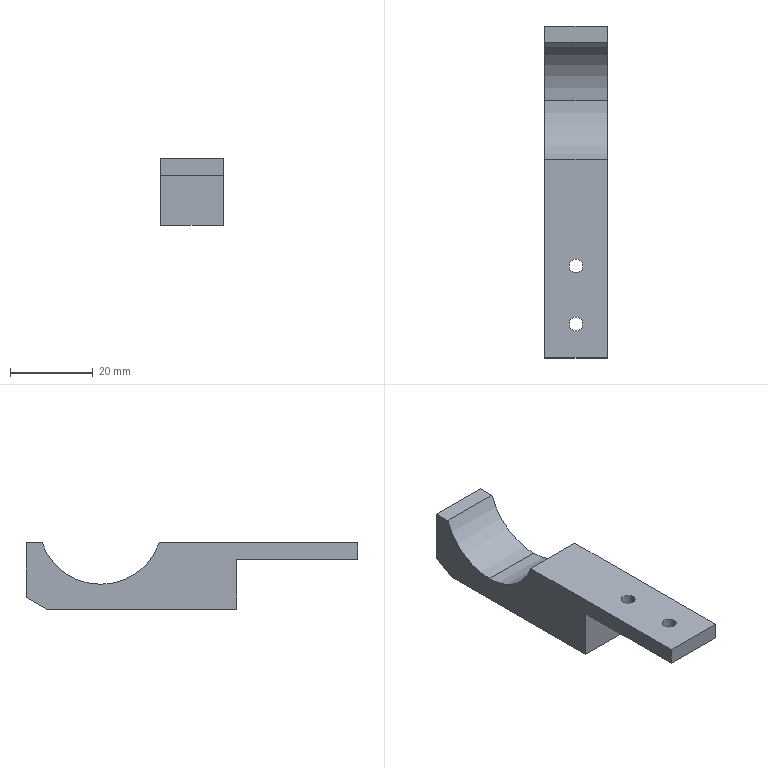Part | SolidWorks | features ICE 2, Chamfer 1, Extrusion 1, HoleWzd 1 | 1 solid | 16 faces | box 15 x 80 x 16 mm | volume 10673 mm3 | plane 10 | cylinder 6 | commonest cylinder face diameters 3.3 x4 30 x2
STEP:
#1=CARTESIAN_POINT('',(-7.5,22.,6.));
#2=VERTEX_POINT('',#1);
#3=CARTESIAN_POINT('',(-7.5,36.142,16.));
#4=VERTEX_POINT('',#3);
#5=CARTESIAN_POINT('',(-7.5,22.,21.));
#6=DIRECTION('',(1.,0.,0.));
#7=DIRECTION('',(0.,0.,-1.));
#8=AXIS2_PLACEMENT_3D('',#5,#6,#7);
#9=CIRCLE('',#8,15.);
#10=EDGE_CURVE('',#2,#4,#9,.T.);
#11=ORIENTED_EDGE('',*,*,#10,.F.);
#12=CARTESIAN_POINT('',(7.5,22.,6.));
#13=VERTEX_POINT('',#12);
#14=CARTESIAN_POINT('',(-7.5,22.,6.));
#15=DIRECTION('',(1.,0.,0.));
#16=VECTOR('',#15,1000.);
#17=LINE('',#14,#16);
#18=EDGE_CURVE('',#2,#13,#17,.T.);
#19=ORIENTED_EDGE('',*,*,#18,.T.);
#20=CARTESIAN_POINT('',(7.5,36.142,16.));
#21=VERTEX_POINT('',#20);
#22=CARTESIAN_POINT('',(7.5,22.,21.));
#23=DIRECTION('',(1.,0.,0.));
#24=DIRECTION('',(0.,0.,-1.));
#25=AXIS2_PLACEMENT_3D('',#22,#23,#24);
#26=CIRCLE('',#25,15.);
#27=EDGE_CURVE('',#13,#21,#26,.T.);
#28=ORIENTED_EDGE('',*,*,#27,.T.);
#29=CARTESIAN_POINT('',(-7.5,36.142,16.));
#30=DIRECTION('',(1.,0.,0.));
#31=VECTOR('',#30,1000.);
#32=LINE('',#29,#31);
#33=EDGE_CURVE('',#4,#21,#32,.T.);
#34=ORIENTED_EDGE('',*,*,#33,.F.);
#35=EDGE_LOOP('',(#11,#19,#28,#34));
#36=FACE_OUTER_BOUND('',#35,.T.);
#37=CARTESIAN_POINT('',(-7.5,22.,21.));
#38=DIRECTION('',(1.,0.,0.));
#39=DIRECTION('',(0.,0.,-1.));
#40=AXIS2_PLACEMENT_3D('',#37,#38,#39);
#41=CYLINDRICAL_SURFACE('',#40,15.);
#42=ADVANCED_FACE('',(#36),#41,.F.);
#43=CARTESIAN_POINT('',(1.65,-17.8,16.));
#44=VERTEX_POINT('',#43);
#45=CARTESIAN_POINT('',(-1.65,-17.8,16.));
#46=VERTEX_POINT('',#45);
#47=CARTESIAN_POINT('',(0.,-17.8,16.));
#48=DIRECTION('',(0.,0.,-1.));
#49=DIRECTION('',(-1.,0.,0.));
#50=AXIS2_PLACEMENT_3D('',#47,#48,#49);
#51=CIRCLE('',#50,1.65);
#52=EDGE_CURVE('',#44,#46,#51,.T.);
#53=ORIENTED_EDGE('',*,*,#52,.F.);
#54=CARTESIAN_POINT('',(1.65,-17.8,12.));
#55=VERTEX_POINT('',#54);
#56=CARTESIAN_POINT('',(1.65,-17.8,12.));
#57=DIRECTION('',(0.,0.,-1.));
#58=VECTOR('',#57,1000.);
#59=LINE('',#56,#58);
#60=EDGE_CURVE('',#44,#55,#59,.T.);
#61=ORIENTED_EDGE('',*,*,#60,.T.);
#62=CARTESIAN_POINT('',(-1.65,-17.8,12.));
#63=VERTEX_POINT('',#62);
#64=CARTESIAN_POINT('',(0.,-17.8,12.));
#65=DIRECTION('',(0.,0.,-1.));
#66=DIRECTION('',(-1.,0.,0.));
#67=AXIS2_PLACEMENT_3D('',#64,#65,#66);
#68=CIRCLE('',#67,1.65);
#69=EDGE_CURVE('',#55,#63,#68,.T.);
#70=ORIENTED_EDGE('',*,*,#69,.T.);
#71=CARTESIAN_POINT('',(-1.65,-17.8,12.));
#72=DIRECTION('',(0.,0.,-1.));
#73=VECTOR('',#72,1000.);
#74=LINE('',#71,#73);
#75=EDGE_CURVE('',#46,#63,#74,.T.);
#76=ORIENTED_EDGE('',*,*,#75,.F.);
#77=EDGE_LOOP('',(#53,#61,#70,#76));
#78=FACE_OUTER_BOUND('',#77,.T.);
#79=CARTESIAN_POINT('',(0.,-17.8,12.));
#80=DIRECTION('',(0.,0.,-1.));
#81=DIRECTION('',(-1.,0.,0.));
#82=AXIS2_PLACEMENT_3D('',#79,#80,#81);
#83=CYLINDRICAL_SURFACE('',#82,1.65);
#84=ADVANCED_FACE('',(#78),#83,.F.);
#85=CARTESIAN_POINT('',(1.65,-31.8,16.));
#86=VERTEX_POINT('',#85);
#87=CARTESIAN_POINT('',(-1.65,-31.8,16.));
#88=VERTEX_POINT('',#87);
#89=CARTESIAN_POINT('',(0.,-31.8,16.));
#90=DIRECTION('',(0.,0.,-1.));
#91=DIRECTION('',(-1.,0.,0.));
#92=AXIS2_PLACEMENT_3D('',#89,#90,#91);
#93=CIRCLE('',#92,1.65);
#94=EDGE_CURVE('',#86,#88,#93,.T.);
#95=ORIENTED_EDGE('',*,*,#94,.F.);
#96=CARTESIAN_POINT('',(1.65,-31.8,12.));
#97=VERTEX_POINT('',#96);
#98=CARTESIAN_POINT('',(1.65,-31.8,12.));
#99=DIRECTION('',(0.,0.,-1.));
#100=VECTOR('',#99,1000.);
#101=LINE('',#98,#100);
#102=EDGE_CURVE('',#86,#97,#101,.T.);
#103=ORIENTED_EDGE('',*,*,#102,.T.);
#104=CARTESIAN_POINT('',(-1.65,-31.8,12.));
#105=VERTEX_POINT('',#104);
#106=CARTESIAN_POINT('',(0.,-31.8,12.));
#107=DIRECTION('',(0.,0.,-1.));
#108=DIRECTION('',(-1.,0.,0.));
#109=AXIS2_PLACEMENT_3D('',#106,#107,#108);
#110=CIRCLE('',#109,1.65);
#111=EDGE_CURVE('',#97,#105,#110,.T.);
#112=ORIENTED_EDGE('',*,*,#111,.T.);
#113=CARTESIAN_POINT('',(-1.65,-31.8,12.));
#114=DIRECTION('',(0.,0.,-1.));
#115=VECTOR('',#114,1000.);
#116=LINE('',#113,#115);
#117=EDGE_CURVE('',#88,#105,#116,.T.);
#118=ORIENTED_EDGE('',*,*,#117,.F.);
#119=EDGE_LOOP('',(#95,#103,#112,#118));
#120=FACE_OUTER_BOUND('',#119,.T.);
#121=CARTESIAN_POINT('',(0.,-31.8,12.));
#122=DIRECTION('',(0.,0.,-1.));
#123=DIRECTION('',(-1.,0.,0.));
#124=AXIS2_PLACEMENT_3D('',#121,#122,#123);
#125=CYLINDRICAL_SURFACE('',#124,1.65);
#126=ADVANCED_FACE('',(#120),#125,.F.);
#127=CARTESIAN_POINT('',(-7.5,40.,16.));
#128=VERTEX_POINT('',#127);
#129=CARTESIAN_POINT('',(-7.5,-40.,16.));
#130=DIRECTION('',(0.,-1.,0.));
#131=VECTOR('',#130,1000.);
#132=LINE('',#129,#131);
#133=EDGE_CURVE('',#128,#4,#132,.T.);
#134=ORIENTED_EDGE('',*,*,#133,.T.);
#135=ORIENTED_EDGE('',*,*,#33,.T.);
#136=CARTESIAN_POINT('',(7.5,40.,16.));
#137=VERTEX_POINT('',#136);
#138=CARTESIAN_POINT('',(7.5,-40.,16.));
#139=DIRECTION('',(0.,1.,0.));
#140=VECTOR('',#139,1000.);
#141=LINE('',#138,#140);
#142=EDGE_CURVE('',#21,#137,#141,.T.);
#143=ORIENTED_EDGE('',*,*,#142,.T.);
#144=CARTESIAN_POINT('',(-7.5,40.,16.));
#145=DIRECTION('',(-1.,0.,0.));
#146=VECTOR('',#145,1000.);
#147=LINE('',#144,#146);
#148=EDGE_CURVE('',#137,#128,#147,.T.);
#149=ORIENTED_EDGE('',*,*,#148,.T.);
#150=EDGE_LOOP('',(#134,#135,#143,#149));
#151=FACE_OUTER_BOUND('',#150,.T.);
#152=CARTESIAN_POINT('',(0.,0.,16.));
#153=DIRECTION('',(0.,0.,-1.));
#154=DIRECTION('',(-1.,0.,0.));
#155=AXIS2_PLACEMENT_3D('',#152,#153,#154);
#156=PLANE('',#155);
#157=ADVANCED_FACE('',(#151),#156,.F.);
#158=ORIENTED_EDGE('',*,*,#142,.F.);
#159=ORIENTED_EDGE('',*,*,#27,.F.);
#160=CARTESIAN_POINT('',(7.5,7.858,16.));
#161=VERTEX_POINT('',#160);
#162=CARTESIAN_POINT('',(7.5,22.,21.));
#163=DIRECTION('',(1.,0.,0.));
#164=DIRECTION('',(0.,0.,-1.));
#165=AXIS2_PLACEMENT_3D('',#162,#163,#164);
#166=CIRCLE('',#165,15.);
#167=EDGE_CURVE('',#161,#13,#166,.T.);
#168=ORIENTED_EDGE('',*,*,#167,.F.);
#169=CARTESIAN_POINT('',(7.5,-40.,16.));
#170=VERTEX_POINT('',#169);
#171=CARTESIAN_POINT('',(7.5,-40.,16.));
#172=DIRECTION('',(0.,1.,0.));
#173=VECTOR('',#172,1000.);
#174=LINE('',#171,#173);
#175=EDGE_CURVE('',#170,#161,#174,.T.);
#176=ORIENTED_EDGE('',*,*,#175,.F.);
#177=CARTESIAN_POINT('',(7.5,-40.,12.));
#178=VERTEX_POINT('',#177);
#179=CARTESIAN_POINT('',(7.5,-40.,16.));
#180=DIRECTION('',(0.,0.,-1.));
#181=VECTOR('',#180,1000.);
#182=LINE('',#179,#181);
#183=EDGE_CURVE('',#170,#178,#182,.T.);
#184=ORIENTED_EDGE('',*,*,#183,.T.);
#185=CARTESIAN_POINT('',(7.5,-10.8,12.));
#186=VERTEX_POINT('',#185);
#187=CARTESIAN_POINT('',(7.5,-40.,12.));
#188=DIRECTION('',(0.,-1.,0.));
#189=VECTOR('',#188,1000.);
#190=LINE('',#187,#189);
#191=EDGE_CURVE('',#186,#178,#190,.T.);
#192=ORIENTED_EDGE('',*,*,#191,.F.);
#193=CARTESIAN_POINT('',(7.5,-10.8,0.));
#194=VERTEX_POINT('',#193);
#195=CARTESIAN_POINT('',(7.5,-10.8,12.));
#196=DIRECTION('',(0.,0.,1.));
#197=VECTOR('',#196,1000.);
#198=LINE('',#195,#197);
#199=EDGE_CURVE('',#194,#186,#198,.T.);
#200=ORIENTED_EDGE('',*,*,#199,.F.);
#201=CARTESIAN_POINT('',(7.5,35.,0.));
#202=VERTEX_POINT('',#201);
#203=CARTESIAN_POINT('',(7.5,-40.,0.));
#204=DIRECTION('',(0.,1.,0.));
#205=VECTOR('',#204,1000.);
#206=LINE('',#203,#205);
#207=EDGE_CURVE('',#194,#202,#206,.T.);
#208=ORIENTED_EDGE('',*,*,#207,.T.);
#209=CARTESIAN_POINT('',(7.5,40.,2.887));
#210=VERTEX_POINT('',#209);
#211=CARTESIAN_POINT('',(7.5,40.,2.887));
#212=DIRECTION('',(0.,0.866,0.5));
#213=VECTOR('',#212,1000.);
#214=LINE('',#211,#213);
#215=EDGE_CURVE('',#202,#210,#214,.T.);
#216=ORIENTED_EDGE('',*,*,#215,.T.);
#217=CARTESIAN_POINT('',(7.5,40.,16.));
#218=DIRECTION('',(0.,0.,-1.));
#219=VECTOR('',#218,1000.);
#220=LINE('',#217,#219);
#221=EDGE_CURVE('',#137,#210,#220,.T.);
#222=ORIENTED_EDGE('',*,*,#221,.F.);
#223=EDGE_LOOP('',(#158,#159,#168,#176,#184,#192,#200,#208,#216,#222));
#224=FACE_OUTER_BOUND('',#223,.T.);
#225=CARTESIAN_POINT('',(7.5,-40.,16.));
#226=DIRECTION('',(-1.,0.,0.));
#227=DIRECTION('',(0.,0.,1.));
#228=AXIS2_PLACEMENT_3D('',#225,#226,#227);
#229=PLANE('',#228);
#230=ADVANCED_FACE('',(#224),#229,.F.);
#231=ORIENTED_EDGE('',*,*,#221,.T.);
#232=CARTESIAN_POINT('',(-7.5,40.,2.887));
#233=VERTEX_POINT('',#232);
#234=CARTESIAN_POINT('',(-7.5,40.,2.887));
#235=DIRECTION('',(-1.,0.,0.));
#236=VECTOR('',#235,1000.);
#237=LINE('',#234,#236);
#238=EDGE_CURVE('',#210,#233,#237,.T.);
#239=ORIENTED_EDGE('',*,*,#238,.T.);
#240=CARTESIAN_POINT('',(-7.5,40.,16.));
#241=DIRECTION('',(0.,0.,-1.));
#242=VECTOR('',#241,1000.);
#243=LINE('',#240,#242);
#244=EDGE_CURVE('',#128,#233,#243,.T.);
#245=ORIENTED_EDGE('',*,*,#244,.F.);
#246=ORIENTED_EDGE('',*,*,#148,.F.);
#247=EDGE_LOOP('',(#231,#239,#245,#246));
#248=FACE_OUTER_BOUND('',#247,.T.);
#249=CARTESIAN_POINT('',(-7.5,40.,16.));
#250=DIRECTION('',(0.,-1.,0.));
#251=DIRECTION('',(0.,0.,-1.));
#252=AXIS2_PLACEMENT_3D('',#249,#250,#251);
#253=PLANE('',#252);
#254=ADVANCED_FACE('',(#248),#253,.F.);
#255=CARTESIAN_POINT('',(-7.5,7.858,16.));
#256=VERTEX_POINT('',#255);
#257=CARTESIAN_POINT('',(-7.5,-40.,16.));
#258=VERTEX_POINT('',#257);
#259=CARTESIAN_POINT('',(-7.5,-40.,16.));
#260=DIRECTION('',(0.,-1.,0.));
#261=VECTOR('',#260,1000.);
#262=LINE('',#259,#261);
#263=EDGE_CURVE('',#256,#258,#262,.T.);
#264=ORIENTED_EDGE('',*,*,#263,.F.);
#265=CARTESIAN_POINT('',(-7.5,22.,21.));
#266=DIRECTION('',(1.,0.,0.));
#267=DIRECTION('',(0.,0.,-1.));
#268=AXIS2_PLACEMENT_3D('',#265,#266,#267);
#269=CIRCLE('',#268,15.);
#270=EDGE_CURVE('',#256,#2,#269,.T.);
#271=ORIENTED_EDGE('',*,*,#270,.T.);
#272=ORIENTED_EDGE('',*,*,#10,.T.);
#273=ORIENTED_EDGE('',*,*,#133,.F.);
#274=ORIENTED_EDGE('',*,*,#244,.T.);
#275=CARTESIAN_POINT('',(-7.5,35.,0.));
#276=VERTEX_POINT('',#275);
#277=CARTESIAN_POINT('',(-7.5,40.,2.887));
#278=DIRECTION('',(0.,-0.866,-0.5));
#279=VECTOR('',#278,1000.);
#280=LINE('',#277,#279);
#281=EDGE_CURVE('',#233,#276,#280,.T.);
#282=ORIENTED_EDGE('',*,*,#281,.T.);
#283=CARTESIAN_POINT('',(-7.5,-10.8,0.));
#284=VERTEX_POINT('',#283);
#285=CARTESIAN_POINT('',(-7.5,-40.,0.));
#286=DIRECTION('',(0.,-1.,0.));
#287=VECTOR('',#286,1000.);
#288=LINE('',#285,#287);
#289=EDGE_CURVE('',#276,#284,#288,.T.);
#290=ORIENTED_EDGE('',*,*,#289,.T.);
#291=CARTESIAN_POINT('',(-7.5,-10.8,12.));
#292=VERTEX_POINT('',#291);
#293=CARTESIAN_POINT('',(-7.5,-10.8,12.));
#294=DIRECTION('',(0.,0.,1.));
#295=VECTOR('',#294,1000.);
#296=LINE('',#293,#295);
#297=EDGE_CURVE('',#284,#292,#296,.T.);
#298=ORIENTED_EDGE('',*,*,#297,.T.);
#299=CARTESIAN_POINT('',(-7.5,-40.,12.));
#300=VERTEX_POINT('',#299);
#301=CARTESIAN_POINT('',(-7.5,-40.,12.));
#302=DIRECTION('',(0.,-1.,0.));
#303=VECTOR('',#302,1000.);
#304=LINE('',#301,#303);
#305=EDGE_CURVE('',#292,#300,#304,.T.);
#306=ORIENTED_EDGE('',*,*,#305,.T.);
#307=CARTESIAN_POINT('',(-7.5,-40.,16.));
#308=DIRECTION('',(0.,0.,-1.));
#309=VECTOR('',#308,1000.);
#310=LINE('',#307,#309);
#311=EDGE_CURVE('',#258,#300,#310,.T.);
#312=ORIENTED_EDGE('',*,*,#311,.F.);
#313=EDGE_LOOP('',(#264,#271,#272,#273,#274,#282,#290,#298,#306,#312));
#314=FACE_OUTER_BOUND('',#313,.T.);
#315=CARTESIAN_POINT('',(-7.5,-40.,16.));
#316=DIRECTION('',(1.,0.,0.));
#317=DIRECTION('',(0.,0.,-1.));
#318=AXIS2_PLACEMENT_3D('',#315,#316,#317);
#319=PLANE('',#318);
#320=ADVANCED_FACE('',(#314),#319,.F.);
#321=ORIENTED_EDGE('',*,*,#311,.T.);
#322=CARTESIAN_POINT('',(-7.5,-40.,12.));
#323=DIRECTION('',(1.,0.,0.));
#324=VECTOR('',#323,1000.);
#325=LINE('',#322,#324);
#326=EDGE_CURVE('',#300,#178,#325,.T.);
#327=ORIENTED_EDGE('',*,*,#326,.T.);
#328=ORIENTED_EDGE('',*,*,#183,.F.);
#329=CARTESIAN_POINT('',(-7.5,-40.,16.));
#330=DIRECTION('',(1.,0.,0.));
#331=VECTOR('',#330,1000.);
#332=LINE('',#329,#331);
#333=EDGE_CURVE('',#258,#170,#332,.T.);
#334=ORIENTED_EDGE('',*,*,#333,.F.);
#335=EDGE_LOOP('',(#321,#327,#328,#334));
#336=FACE_OUTER_BOUND('',#335,.T.);
#337=CARTESIAN_POINT('',(-7.5,-40.,16.));
#338=DIRECTION('',(0.,1.,0.));
#339=DIRECTION('',(0.,0.,1.));
#340=AXIS2_PLACEMENT_3D('',#337,#338,#339);
#341=PLANE('',#340);
#342=ADVANCED_FACE('',(#336),#341,.F.);
#343=CARTESIAN_POINT('',(0.,-17.8,16.));
#344=DIRECTION('',(0.,0.,-1.));
#345=DIRECTION('',(-1.,0.,0.));
#346=AXIS2_PLACEMENT_3D('',#343,#344,#345);
#347=CIRCLE('',#346,1.65);
#348=EDGE_CURVE('',#46,#44,#347,.T.);
#349=ORIENTED_EDGE('',*,*,#348,.T.);
#350=ORIENTED_EDGE('',*,*,#52,.T.);
#351=EDGE_LOOP('',(#349,#350));
#352=FACE_BOUND('',#351,.T.);
#353=CARTESIAN_POINT('',(0.,-31.8,16.));
#354=DIRECTION('',(0.,0.,-1.));
#355=DIRECTION('',(-1.,0.,0.));
#356=AXIS2_PLACEMENT_3D('',#353,#354,#355);
#357=CIRCLE('',#356,1.65);
#358=EDGE_CURVE('',#88,#86,#357,.T.);
#359=ORIENTED_EDGE('',*,*,#358,.T.);
#360=ORIENTED_EDGE('',*,*,#94,.T.);
#361=EDGE_LOOP('',(#359,#360));
#362=FACE_BOUND('',#361,.T.);
#363=ORIENTED_EDGE('',*,*,#175,.T.);
#364=CARTESIAN_POINT('',(-7.5,7.858,16.));
#365=DIRECTION('',(-1.,0.,0.));
#366=VECTOR('',#365,1000.);
#367=LINE('',#364,#366);
#368=EDGE_CURVE('',#161,#256,#367,.T.);
#369=ORIENTED_EDGE('',*,*,#368,.T.);
#370=ORIENTED_EDGE('',*,*,#263,.T.);
#371=ORIENTED_EDGE('',*,*,#333,.T.);
#372=EDGE_LOOP('',(#363,#369,#370,#371));
#373=FACE_OUTER_BOUND('',#372,.T.);
#374=CARTESIAN_POINT('',(0.,0.,16.));
#375=DIRECTION('',(0.,0.,-1.));
#376=DIRECTION('',(-1.,0.,0.));
#377=AXIS2_PLACEMENT_3D('',#374,#375,#376);
#378=PLANE('',#377);
#379=ADVANCED_FACE('',(#352,#362,#373),#378,.F.);
#380=ORIENTED_EDGE('',*,*,#289,.F.);
#381=CARTESIAN_POINT('',(7.5,35.,0.));
#382=DIRECTION('',(1.,0.,0.));
#383=VECTOR('',#382,1000.);
#384=LINE('',#381,#383);
#385=EDGE_CURVE('',#276,#202,#384,.T.);
#386=ORIENTED_EDGE('',*,*,#385,.T.);
#387=ORIENTED_EDGE('',*,*,#207,.F.);
#388=CARTESIAN_POINT('',(-7.5,-10.8,0.));
#389=DIRECTION('',(1.,0.,0.));
#390=VECTOR('',#389,1000.);
#391=LINE('',#388,#390);
#392=EDGE_CURVE('',#284,#194,#391,.T.);
#393=ORIENTED_EDGE('',*,*,#392,.F.);
#394=EDGE_LOOP('',(#380,#386,#387,#393));
#395=FACE_OUTER_BOUND('',#394,.T.);
#396=CARTESIAN_POINT('',(0.,0.,0.));
#397=DIRECTION('',(0.,0.,-1.));
#398=DIRECTION('',(-1.,0.,0.));
#399=AXIS2_PLACEMENT_3D('',#396,#397,#398);
#400=PLANE('',#399);
#401=ADVANCED_FACE('',(#395),#400,.T.);
#402=CARTESIAN_POINT('',(0.,-17.8,12.));
#403=DIRECTION('',(0.,0.,-1.));
#404=DIRECTION('',(-1.,0.,0.));
#405=AXIS2_PLACEMENT_3D('',#402,#403,#404);
#406=CIRCLE('',#405,1.65);
#407=EDGE_CURVE('',#63,#55,#406,.T.);
#408=ORIENTED_EDGE('',*,*,#407,.F.);
#409=ORIENTED_EDGE('',*,*,#69,.F.);
#410=EDGE_LOOP('',(#408,#409));
#411=FACE_BOUND('',#410,.T.);
#412=CARTESIAN_POINT('',(0.,-31.8,12.));
#413=DIRECTION('',(0.,0.,-1.));
#414=DIRECTION('',(-1.,0.,0.));
#415=AXIS2_PLACEMENT_3D('',#412,#413,#414);
#416=CIRCLE('',#415,1.65);
#417=EDGE_CURVE('',#105,#97,#416,.T.);
#418=ORIENTED_EDGE('',*,*,#417,.F.);
#419=ORIENTED_EDGE('',*,*,#111,.F.);
#420=EDGE_LOOP('',(#418,#419));
#421=FACE_BOUND('',#420,.T.);
#422=ORIENTED_EDGE('',*,*,#191,.T.);
#423=ORIENTED_EDGE('',*,*,#326,.F.);
#424=ORIENTED_EDGE('',*,*,#305,.F.);
#425=CARTESIAN_POINT('',(-7.5,-10.8,12.));
#426=DIRECTION('',(1.,0.,0.));
#427=VECTOR('',#426,1000.);
#428=LINE('',#425,#427);
#429=EDGE_CURVE('',#292,#186,#428,.T.);
#430=ORIENTED_EDGE('',*,*,#429,.T.);
#431=EDGE_LOOP('',(#422,#423,#424,#430));
#432=FACE_OUTER_BOUND('',#431,.T.);
#433=CARTESIAN_POINT('',(-7.5,-40.,12.));
#434=DIRECTION('',(0.,0.,1.));
#435=DIRECTION('',(1.,0.,0.));
#436=AXIS2_PLACEMENT_3D('',#433,#434,#435);
#437=PLANE('',#436);
#438=ADVANCED_FACE('',(#411,#421,#432),#437,.F.);
#439=ORIENTED_EDGE('',*,*,#199,.T.);
#440=ORIENTED_EDGE('',*,*,#429,.F.);
#441=ORIENTED_EDGE('',*,*,#297,.F.);
#442=ORIENTED_EDGE('',*,*,#392,.T.);
#443=EDGE_LOOP('',(#439,#440,#441,#442));
#444=FACE_OUTER_BOUND('',#443,.T.);
#445=CARTESIAN_POINT('',(-7.5,-10.8,12.));
#446=DIRECTION('',(0.,1.,0.));
#447=DIRECTION('',(0.,0.,1.));
#448=AXIS2_PLACEMENT_3D('',#445,#446,#447);
#449=PLANE('',#448);
#450=ADVANCED_FACE('',(#444),#449,.F.);
#451=ORIENTED_EDGE('',*,*,#102,.F.);
#452=ORIENTED_EDGE('',*,*,#358,.F.);
#453=ORIENTED_EDGE('',*,*,#117,.T.);
#454=ORIENTED_EDGE('',*,*,#417,.T.);
#455=EDGE_LOOP('',(#451,#452,#453,#454));
#456=FACE_OUTER_BOUND('',#455,.T.);
#457=CARTESIAN_POINT('',(0.,-31.8,12.));
#458=DIRECTION('',(0.,0.,-1.));
#459=DIRECTION('',(-1.,0.,0.));
#460=AXIS2_PLACEMENT_3D('',#457,#458,#459);
#461=CYLINDRICAL_SURFACE('',#460,1.65);
#462=ADVANCED_FACE('',(#456),#461,.F.);
#463=ORIENTED_EDGE('',*,*,#60,.F.);
#464=ORIENTED_EDGE('',*,*,#348,.F.);
#465=ORIENTED_EDGE('',*,*,#75,.T.);
#466=ORIENTED_EDGE('',*,*,#407,.T.);
#467=EDGE_LOOP('',(#463,#464,#465,#466));
#468=FACE_OUTER_BOUND('',#467,.T.);
#469=CARTESIAN_POINT('',(0.,-17.8,12.));
#470=DIRECTION('',(0.,0.,-1.));
#471=DIRECTION('',(-1.,0.,0.));
#472=AXIS2_PLACEMENT_3D('',#469,#470,#471);
#473=CYLINDRICAL_SURFACE('',#472,1.65);
#474=ADVANCED_FACE('',(#468),#473,.F.);
#475=ORIENTED_EDGE('',*,*,#215,.F.);
#476=ORIENTED_EDGE('',*,*,#385,.F.);
#477=ORIENTED_EDGE('',*,*,#281,.F.);
#478=ORIENTED_EDGE('',*,*,#238,.F.);
#479=EDGE_LOOP('',(#475,#476,#477,#478));
#480=FACE_OUTER_BOUND('',#479,.T.);
#481=CARTESIAN_POINT('',(-7.5,40.,2.887));
#482=DIRECTION('',(0.,0.5,-0.866));
#483=DIRECTION('',(1.,0.,0.));
#484=AXIS2_PLACEMENT_3D('',#481,#482,#483);
#485=PLANE('',#484);
#486=ADVANCED_FACE('',(#480),#485,.T.);
#487=ORIENTED_EDGE('',*,*,#18,.F.);
#488=ORIENTED_EDGE('',*,*,#270,.F.);
#489=ORIENTED_EDGE('',*,*,#368,.F.);
#490=ORIENTED_EDGE('',*,*,#167,.T.);
#491=EDGE_LOOP('',(#487,#488,#489,#490));
#492=FACE_OUTER_BOUND('',#491,.T.);
#493=CARTESIAN_POINT('',(-7.5,22.,21.));
#494=DIRECTION('',(1.,0.,0.));
#495=DIRECTION('',(0.,0.,-1.));
#496=AXIS2_PLACEMENT_3D('',#493,#494,#495);
#497=CYLINDRICAL_SURFACE('',#496,15.);
#498=ADVANCED_FACE('',(#492),#497,.F.);
#499=CLOSED_SHELL('',(#42,#84,#126,#157,#230,#254,#320,#342,#379,#401,#438,#450,#462,#474,#486,#498));
#500=MANIFOLD_SOLID_BREP('',#499);
#501=CARTESIAN_POINT('',(0.,0.,0.));
#502=DIRECTION('',(0.,0.,1.));
#503=DIRECTION('',(1.,0.,0.));
#504=AXIS2_PLACEMENT_3D('',#501,#502,#503);
#505=(LENGTH_UNIT()NAMED_UNIT(*)SI_UNIT(.MILLI.,.METRE.));
#506=UNCERTAINTY_MEASURE_WITH_UNIT(LENGTH_MEASURE(0.00001),#505,'','');
#507=(NAMED_UNIT(*)PLANE_ANGLE_UNIT()SI_UNIT($,.RADIAN.));
#508=(NAMED_UNIT(*)SI_UNIT($,.STERADIAN.)SOLID_ANGLE_UNIT());
#509=(GEOMETRIC_REPRESENTATION_CONTEXT(3)GLOBAL_UNCERTAINTY_ASSIGNED_CONTEXT((#506))GLOBAL_UNIT_ASSIGNED_CONTEXT((#505,#507,#508))REPRESENTATION_CONTEXT('',''));
#510=ADVANCED_BREP_SHAPE_REPRESENTATION('',(#500,#504),#509);